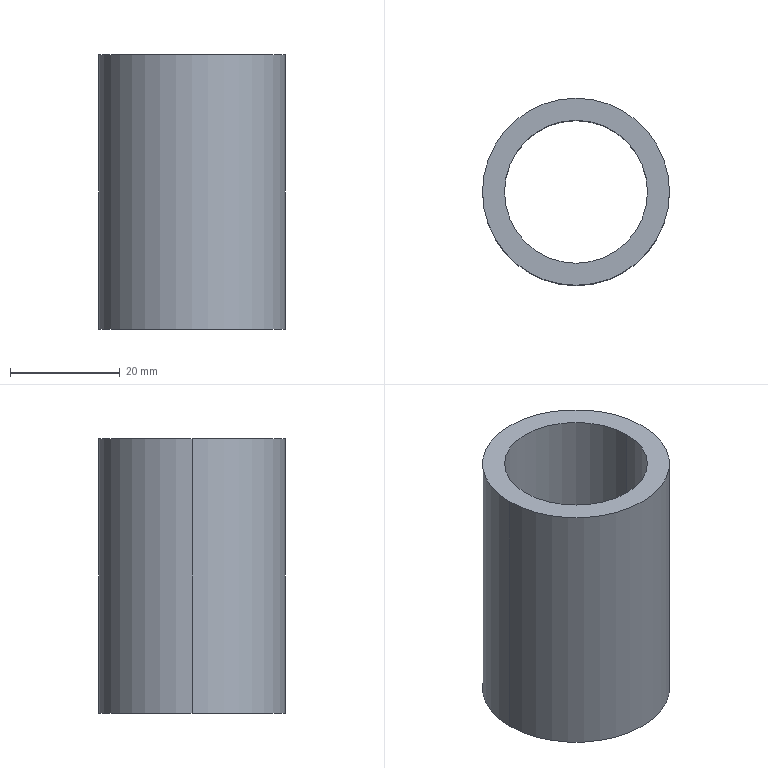Part | SolidWorks | features Extrusion 1 | 1 solid | 6 faces | box 34 x 34 x 50 mm | volume 18850 mm3 | cylinder 4 | plane 2 | commonest cylinder face diameters 26 x2 34 x2
STEP:
#1=CARTESIAN_POINT('',(-13.,0.,50.));
#2=VERTEX_POINT('',#1);
#3=CARTESIAN_POINT('',(13.,0.,50.));
#4=VERTEX_POINT('',#3);
#5=CARTESIAN_POINT('',(0.,0.,50.));
#6=DIRECTION('',(0.,0.,1.));
#7=DIRECTION('',(1.,0.,0.));
#8=AXIS2_PLACEMENT_3D('',#5,#6,#7);
#9=CIRCLE('',#8,13.);
#10=EDGE_CURVE('',#2,#4,#9,.T.);
#11=ORIENTED_EDGE('',*,*,#10,.T.);
#12=CARTESIAN_POINT('',(13.,0.,0.));
#13=VERTEX_POINT('',#12);
#14=CARTESIAN_POINT('',(13.,0.,50.));
#15=DIRECTION('',(0.,0.,-1.));
#16=VECTOR('',#15,1000.);
#17=LINE('',#14,#16);
#18=EDGE_CURVE('',#4,#13,#17,.T.);
#19=ORIENTED_EDGE('',*,*,#18,.T.);
#20=CARTESIAN_POINT('',(-13.,0.,0.));
#21=VERTEX_POINT('',#20);
#22=CARTESIAN_POINT('',(0.,0.,0.));
#23=DIRECTION('',(0.,0.,1.));
#24=DIRECTION('',(1.,0.,0.));
#25=AXIS2_PLACEMENT_3D('',#22,#23,#24);
#26=CIRCLE('',#25,13.);
#27=EDGE_CURVE('',#21,#13,#26,.T.);
#28=ORIENTED_EDGE('',*,*,#27,.F.);
#29=CARTESIAN_POINT('',(-13.,0.,50.));
#30=DIRECTION('',(0.,0.,-1.));
#31=VECTOR('',#30,1000.);
#32=LINE('',#29,#31);
#33=EDGE_CURVE('',#2,#21,#32,.T.);
#34=ORIENTED_EDGE('',*,*,#33,.F.);
#35=EDGE_LOOP('',(#11,#19,#28,#34));
#36=FACE_OUTER_BOUND('',#35,.T.);
#37=CARTESIAN_POINT('',(0.,0.,50.));
#38=DIRECTION('',(0.,0.,-1.));
#39=DIRECTION('',(-1.,0.,0.));
#40=AXIS2_PLACEMENT_3D('',#37,#38,#39);
#41=CYLINDRICAL_SURFACE('',#40,13.);
#42=ADVANCED_FACE('',(#36),#41,.F.);
#43=CARTESIAN_POINT('',(17.,0.,50.));
#44=VERTEX_POINT('',#43);
#45=CARTESIAN_POINT('',(-17.,0.,50.));
#46=VERTEX_POINT('',#45);
#47=CARTESIAN_POINT('',(0.,0.,50.));
#48=DIRECTION('',(0.,0.,1.));
#49=DIRECTION('',(1.,0.,0.));
#50=AXIS2_PLACEMENT_3D('',#47,#48,#49);
#51=CIRCLE('',#50,17.);
#52=EDGE_CURVE('',#44,#46,#51,.T.);
#53=ORIENTED_EDGE('',*,*,#52,.F.);
#54=CARTESIAN_POINT('',(17.,0.,0.));
#55=VERTEX_POINT('',#54);
#56=CARTESIAN_POINT('',(17.,0.,50.));
#57=DIRECTION('',(0.,0.,-1.));
#58=VECTOR('',#57,1000.);
#59=LINE('',#56,#58);
#60=EDGE_CURVE('',#44,#55,#59,.T.);
#61=ORIENTED_EDGE('',*,*,#60,.T.);
#62=CARTESIAN_POINT('',(-17.,0.,0.));
#63=VERTEX_POINT('',#62);
#64=CARTESIAN_POINT('',(0.,0.,0.));
#65=DIRECTION('',(0.,0.,1.));
#66=DIRECTION('',(1.,0.,0.));
#67=AXIS2_PLACEMENT_3D('',#64,#65,#66);
#68=CIRCLE('',#67,17.);
#69=EDGE_CURVE('',#55,#63,#68,.T.);
#70=ORIENTED_EDGE('',*,*,#69,.T.);
#71=CARTESIAN_POINT('',(-17.,0.,50.));
#72=DIRECTION('',(0.,0.,-1.));
#73=VECTOR('',#72,1000.);
#74=LINE('',#71,#73);
#75=EDGE_CURVE('',#46,#63,#74,.T.);
#76=ORIENTED_EDGE('',*,*,#75,.F.);
#77=EDGE_LOOP('',(#53,#61,#70,#76));
#78=FACE_OUTER_BOUND('',#77,.T.);
#79=CARTESIAN_POINT('',(0.,0.,50.));
#80=DIRECTION('',(0.,0.,-1.));
#81=DIRECTION('',(-1.,0.,0.));
#82=AXIS2_PLACEMENT_3D('',#79,#80,#81);
#83=CYLINDRICAL_SURFACE('',#82,17.);
#84=ADVANCED_FACE('',(#78),#83,.T.);
#85=CARTESIAN_POINT('',(0.,0.,50.));
#86=DIRECTION('',(0.,0.,1.));
#87=DIRECTION('',(1.,0.,0.));
#88=AXIS2_PLACEMENT_3D('',#85,#86,#87);
#89=CIRCLE('',#88,17.);
#90=EDGE_CURVE('',#46,#44,#89,.T.);
#91=ORIENTED_EDGE('',*,*,#90,.T.);
#92=ORIENTED_EDGE('',*,*,#52,.T.);
#93=EDGE_LOOP('',(#91,#92));
#94=FACE_OUTER_BOUND('',#93,.T.);
#95=ORIENTED_EDGE('',*,*,#10,.F.);
#96=CARTESIAN_POINT('',(0.,0.,50.));
#97=DIRECTION('',(0.,0.,1.));
#98=DIRECTION('',(1.,0.,0.));
#99=AXIS2_PLACEMENT_3D('',#96,#97,#98);
#100=CIRCLE('',#99,13.);
#101=EDGE_CURVE('',#4,#2,#100,.T.);
#102=ORIENTED_EDGE('',*,*,#101,.F.);
#103=EDGE_LOOP('',(#95,#102));
#104=FACE_BOUND('',#103,.T.);
#105=CARTESIAN_POINT('',(0.,0.,50.));
#106=DIRECTION('',(0.,0.,1.));
#107=DIRECTION('',(1.,0.,0.));
#108=AXIS2_PLACEMENT_3D('',#105,#106,#107);
#109=PLANE('',#108);
#110=ADVANCED_FACE('',(#94,#104),#109,.T.);
#111=CARTESIAN_POINT('',(0.,0.,0.));
#112=DIRECTION('',(0.,0.,1.));
#113=DIRECTION('',(1.,0.,0.));
#114=AXIS2_PLACEMENT_3D('',#111,#112,#113);
#115=CIRCLE('',#114,17.);
#116=EDGE_CURVE('',#63,#55,#115,.T.);
#117=ORIENTED_EDGE('',*,*,#116,.F.);
#118=ORIENTED_EDGE('',*,*,#69,.F.);
#119=EDGE_LOOP('',(#117,#118));
#120=FACE_OUTER_BOUND('',#119,.T.);
#121=ORIENTED_EDGE('',*,*,#27,.T.);
#122=CARTESIAN_POINT('',(0.,0.,0.));
#123=DIRECTION('',(0.,0.,1.));
#124=DIRECTION('',(1.,0.,0.));
#125=AXIS2_PLACEMENT_3D('',#122,#123,#124);
#126=CIRCLE('',#125,13.);
#127=EDGE_CURVE('',#13,#21,#126,.T.);
#128=ORIENTED_EDGE('',*,*,#127,.T.);
#129=EDGE_LOOP('',(#121,#128));
#130=FACE_BOUND('',#129,.T.);
#131=CARTESIAN_POINT('',(0.,0.,0.));
#132=DIRECTION('',(0.,0.,1.));
#133=DIRECTION('',(1.,0.,0.));
#134=AXIS2_PLACEMENT_3D('',#131,#132,#133);
#135=PLANE('',#134);
#136=ADVANCED_FACE('',(#120,#130),#135,.F.);
#137=ORIENTED_EDGE('',*,*,#60,.F.);
#138=ORIENTED_EDGE('',*,*,#90,.F.);
#139=ORIENTED_EDGE('',*,*,#75,.T.);
#140=ORIENTED_EDGE('',*,*,#116,.T.);
#141=EDGE_LOOP('',(#137,#138,#139,#140));
#142=FACE_OUTER_BOUND('',#141,.T.);
#143=CARTESIAN_POINT('',(0.,0.,50.));
#144=DIRECTION('',(0.,0.,-1.));
#145=DIRECTION('',(-1.,0.,0.));
#146=AXIS2_PLACEMENT_3D('',#143,#144,#145);
#147=CYLINDRICAL_SURFACE('',#146,17.);
#148=ADVANCED_FACE('',(#142),#147,.T.);
#149=ORIENTED_EDGE('',*,*,#18,.F.);
#150=ORIENTED_EDGE('',*,*,#101,.T.);
#151=ORIENTED_EDGE('',*,*,#33,.T.);
#152=ORIENTED_EDGE('',*,*,#127,.F.);
#153=EDGE_LOOP('',(#149,#150,#151,#152));
#154=FACE_OUTER_BOUND('',#153,.T.);
#155=CARTESIAN_POINT('',(0.,0.,50.));
#156=DIRECTION('',(0.,0.,-1.));
#157=DIRECTION('',(-1.,0.,0.));
#158=AXIS2_PLACEMENT_3D('',#155,#156,#157);
#159=CYLINDRICAL_SURFACE('',#158,13.);
#160=ADVANCED_FACE('',(#154),#159,.F.);
#161=CLOSED_SHELL('',(#42,#84,#110,#136,#148,#160));
#162=MANIFOLD_SOLID_BREP('',#161);
#163=CARTESIAN_POINT('',(0.,0.,0.));
#164=DIRECTION('',(0.,0.,1.));
#165=DIRECTION('',(1.,0.,0.));
#166=AXIS2_PLACEMENT_3D('',#163,#164,#165);
#167=(LENGTH_UNIT()NAMED_UNIT(*)SI_UNIT(.MILLI.,.METRE.));
#168=UNCERTAINTY_MEASURE_WITH_UNIT(LENGTH_MEASURE(0.00001),#167,'','');
#169=(NAMED_UNIT(*)PLANE_ANGLE_UNIT()SI_UNIT($,.RADIAN.));
#170=(NAMED_UNIT(*)SI_UNIT($,.STERADIAN.)SOLID_ANGLE_UNIT());
#171=(GEOMETRIC_REPRESENTATION_CONTEXT(3)GLOBAL_UNCERTAINTY_ASSIGNED_CONTEXT((#168))GLOBAL_UNIT_ASSIGNED_CONTEXT((#167,#169,#170))REPRESENTATION_CONTEXT('',''));
#172=ADVANCED_BREP_SHAPE_REPRESENTATION('',(#162,#166),#171);